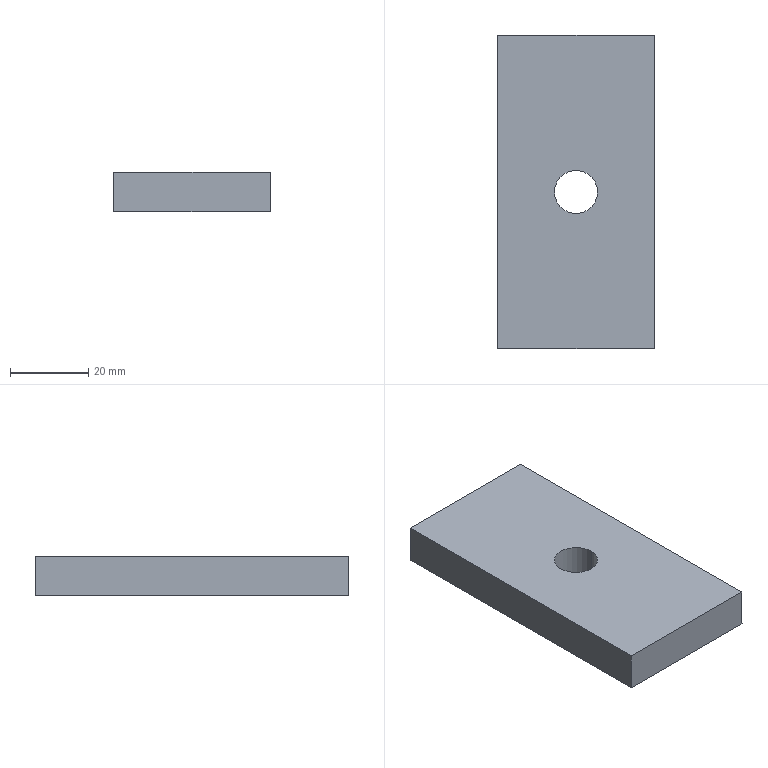Part | SolidWorks | features Extrusion 1, HoleWzd 1 | 1 solid | 8 faces | box 40 x 80 x 10 mm | volume 31050 mm3 | plane 6 | cylinder 2 | commonest cylinder face diameters 11 x2
STEP:
#1=CARTESIAN_POINT('',(14.5,40.,0.));
#2=VERTEX_POINT('',#1);
#3=CARTESIAN_POINT('',(25.5,40.,0.));
#4=VERTEX_POINT('',#3);
#5=CARTESIAN_POINT('',(20.,40.,0.));
#6=DIRECTION('',(0.,0.,1.));
#7=DIRECTION('',(1.,0.,0.));
#8=AXIS2_PLACEMENT_3D('',#5,#6,#7);
#9=CIRCLE('',#8,5.5);
#10=EDGE_CURVE('',#2,#4,#9,.T.);
#11=ORIENTED_EDGE('',*,*,#10,.F.);
#12=CARTESIAN_POINT('',(14.5,40.,10.));
#13=VERTEX_POINT('',#12);
#14=CARTESIAN_POINT('',(14.5,40.,10.));
#15=DIRECTION('',(0.,0.,1.));
#16=VECTOR('',#15,1000.);
#17=LINE('',#14,#16);
#18=EDGE_CURVE('',#2,#13,#17,.T.);
#19=ORIENTED_EDGE('',*,*,#18,.T.);
#20=CARTESIAN_POINT('',(25.5,40.,10.));
#21=VERTEX_POINT('',#20);
#22=CARTESIAN_POINT('',(20.,40.,10.));
#23=DIRECTION('',(0.,0.,1.));
#24=DIRECTION('',(1.,0.,0.));
#25=AXIS2_PLACEMENT_3D('',#22,#23,#24);
#26=CIRCLE('',#25,5.5);
#27=EDGE_CURVE('',#13,#21,#26,.T.);
#28=ORIENTED_EDGE('',*,*,#27,.T.);
#29=CARTESIAN_POINT('',(25.5,40.,10.));
#30=DIRECTION('',(0.,0.,1.));
#31=VECTOR('',#30,1000.);
#32=LINE('',#29,#31);
#33=EDGE_CURVE('',#4,#21,#32,.T.);
#34=ORIENTED_EDGE('',*,*,#33,.F.);
#35=EDGE_LOOP('',(#11,#19,#28,#34));
#36=FACE_OUTER_BOUND('',#35,.T.);
#37=CARTESIAN_POINT('',(20.,40.,10.));
#38=DIRECTION('',(0.,0.,1.));
#39=DIRECTION('',(1.,0.,0.));
#40=AXIS2_PLACEMENT_3D('',#37,#38,#39);
#41=CYLINDRICAL_SURFACE('',#40,5.5);
#42=ADVANCED_FACE('',(#36),#41,.F.);
#43=CARTESIAN_POINT('',(0.,80.,0.));
#44=VERTEX_POINT('',#43);
#45=CARTESIAN_POINT('',(0.,0.,0.));
#46=VERTEX_POINT('',#45);
#47=CARTESIAN_POINT('',(0.,0.,0.));
#48=DIRECTION('',(0.,-1.,0.));
#49=VECTOR('',#48,1000.);
#50=LINE('',#47,#49);
#51=EDGE_CURVE('',#44,#46,#50,.T.);
#52=ORIENTED_EDGE('',*,*,#51,.T.);
#53=CARTESIAN_POINT('',(0.,0.,10.));
#54=VERTEX_POINT('',#53);
#55=CARTESIAN_POINT('',(0.,0.,10.));
#56=DIRECTION('',(0.,0.,-1.));
#57=VECTOR('',#56,1000.);
#58=LINE('',#55,#57);
#59=EDGE_CURVE('',#54,#46,#58,.T.);
#60=ORIENTED_EDGE('',*,*,#59,.F.);
#61=CARTESIAN_POINT('',(0.,80.,10.));
#62=VERTEX_POINT('',#61);
#63=CARTESIAN_POINT('',(0.,0.,10.));
#64=DIRECTION('',(0.,-1.,0.));
#65=VECTOR('',#64,1000.);
#66=LINE('',#63,#65);
#67=EDGE_CURVE('',#62,#54,#66,.T.);
#68=ORIENTED_EDGE('',*,*,#67,.F.);
#69=CARTESIAN_POINT('',(0.,80.,10.));
#70=DIRECTION('',(0.,0.,-1.));
#71=VECTOR('',#70,1000.);
#72=LINE('',#69,#71);
#73=EDGE_CURVE('',#62,#44,#72,.T.);
#74=ORIENTED_EDGE('',*,*,#73,.T.);
#75=EDGE_LOOP('',(#52,#60,#68,#74));
#76=FACE_OUTER_BOUND('',#75,.T.);
#77=CARTESIAN_POINT('',(0.,0.,10.));
#78=DIRECTION('',(1.,0.,0.));
#79=DIRECTION('',(0.,1.,0.));
#80=AXIS2_PLACEMENT_3D('',#77,#78,#79);
#81=PLANE('',#80);
#82=ADVANCED_FACE('',(#76),#81,.F.);
#83=CARTESIAN_POINT('',(40.,0.,0.));
#84=VERTEX_POINT('',#83);
#85=CARTESIAN_POINT('',(0.,0.,0.));
#86=DIRECTION('',(1.,0.,0.));
#87=VECTOR('',#86,1000.);
#88=LINE('',#85,#87);
#89=EDGE_CURVE('',#46,#84,#88,.T.);
#90=ORIENTED_EDGE('',*,*,#89,.T.);
#91=CARTESIAN_POINT('',(40.,0.,10.));
#92=VERTEX_POINT('',#91);
#93=CARTESIAN_POINT('',(40.,0.,10.));
#94=DIRECTION('',(0.,0.,-1.));
#95=VECTOR('',#94,1000.);
#96=LINE('',#93,#95);
#97=EDGE_CURVE('',#92,#84,#96,.T.);
#98=ORIENTED_EDGE('',*,*,#97,.F.);
#99=CARTESIAN_POINT('',(0.,0.,10.));
#100=DIRECTION('',(1.,0.,0.));
#101=VECTOR('',#100,1000.);
#102=LINE('',#99,#101);
#103=EDGE_CURVE('',#54,#92,#102,.T.);
#104=ORIENTED_EDGE('',*,*,#103,.F.);
#105=ORIENTED_EDGE('',*,*,#59,.T.);
#106=EDGE_LOOP('',(#90,#98,#104,#105));
#107=FACE_OUTER_BOUND('',#106,.T.);
#108=CARTESIAN_POINT('',(0.,0.,10.));
#109=DIRECTION('',(0.,1.,0.));
#110=DIRECTION('',(0.,0.,1.));
#111=AXIS2_PLACEMENT_3D('',#108,#109,#110);
#112=PLANE('',#111);
#113=ADVANCED_FACE('',(#107),#112,.F.);
#114=CARTESIAN_POINT('',(40.,80.,0.));
#115=VERTEX_POINT('',#114);
#116=CARTESIAN_POINT('',(40.,0.,0.));
#117=DIRECTION('',(0.,1.,0.));
#118=VECTOR('',#117,1000.);
#119=LINE('',#116,#118);
#120=EDGE_CURVE('',#84,#115,#119,.T.);
#121=ORIENTED_EDGE('',*,*,#120,.T.);
#122=CARTESIAN_POINT('',(40.,80.,10.));
#123=VERTEX_POINT('',#122);
#124=CARTESIAN_POINT('',(40.,80.,10.));
#125=DIRECTION('',(0.,0.,-1.));
#126=VECTOR('',#125,1000.);
#127=LINE('',#124,#126);
#128=EDGE_CURVE('',#123,#115,#127,.T.);
#129=ORIENTED_EDGE('',*,*,#128,.F.);
#130=CARTESIAN_POINT('',(40.,0.,10.));
#131=DIRECTION('',(0.,1.,0.));
#132=VECTOR('',#131,1000.);
#133=LINE('',#130,#132);
#134=EDGE_CURVE('',#92,#123,#133,.T.);
#135=ORIENTED_EDGE('',*,*,#134,.F.);
#136=ORIENTED_EDGE('',*,*,#97,.T.);
#137=EDGE_LOOP('',(#121,#129,#135,#136));
#138=FACE_OUTER_BOUND('',#137,.T.);
#139=CARTESIAN_POINT('',(40.,0.,10.));
#140=DIRECTION('',(-1.,0.,0.));
#141=DIRECTION('',(0.,0.,1.));
#142=AXIS2_PLACEMENT_3D('',#139,#140,#141);
#143=PLANE('',#142);
#144=ADVANCED_FACE('',(#138),#143,.F.);
#145=CARTESIAN_POINT('',(0.,80.,0.));
#146=DIRECTION('',(-1.,0.,0.));
#147=VECTOR('',#146,1000.);
#148=LINE('',#145,#147);
#149=EDGE_CURVE('',#115,#44,#148,.T.);
#150=ORIENTED_EDGE('',*,*,#149,.T.);
#151=ORIENTED_EDGE('',*,*,#73,.F.);
#152=CARTESIAN_POINT('',(0.,80.,10.));
#153=DIRECTION('',(-1.,0.,0.));
#154=VECTOR('',#153,1000.);
#155=LINE('',#152,#154);
#156=EDGE_CURVE('',#123,#62,#155,.T.);
#157=ORIENTED_EDGE('',*,*,#156,.F.);
#158=ORIENTED_EDGE('',*,*,#128,.T.);
#159=EDGE_LOOP('',(#150,#151,#157,#158));
#160=FACE_OUTER_BOUND('',#159,.T.);
#161=CARTESIAN_POINT('',(0.,80.,10.));
#162=DIRECTION('',(0.,-1.,0.));
#163=DIRECTION('',(0.,0.,-1.));
#164=AXIS2_PLACEMENT_3D('',#161,#162,#163);
#165=PLANE('',#164);
#166=ADVANCED_FACE('',(#160),#165,.F.);
#167=CARTESIAN_POINT('',(20.,40.,10.));
#168=DIRECTION('',(0.,0.,1.));
#169=DIRECTION('',(1.,0.,0.));
#170=AXIS2_PLACEMENT_3D('',#167,#168,#169);
#171=CIRCLE('',#170,5.5);
#172=EDGE_CURVE('',#21,#13,#171,.T.);
#173=ORIENTED_EDGE('',*,*,#172,.F.);
#174=ORIENTED_EDGE('',*,*,#27,.F.);
#175=EDGE_LOOP('',(#173,#174));
#176=FACE_BOUND('',#175,.T.);
#177=ORIENTED_EDGE('',*,*,#67,.T.);
#178=ORIENTED_EDGE('',*,*,#103,.T.);
#179=ORIENTED_EDGE('',*,*,#134,.T.);
#180=ORIENTED_EDGE('',*,*,#156,.T.);
#181=EDGE_LOOP('',(#177,#178,#179,#180));
#182=FACE_OUTER_BOUND('',#181,.T.);
#183=CARTESIAN_POINT('',(0.,0.,10.));
#184=DIRECTION('',(0.,0.,-1.));
#185=DIRECTION('',(-1.,0.,0.));
#186=AXIS2_PLACEMENT_3D('',#183,#184,#185);
#187=PLANE('',#186);
#188=ADVANCED_FACE('',(#176,#182),#187,.F.);
#189=CARTESIAN_POINT('',(20.,40.,0.));
#190=DIRECTION('',(0.,0.,1.));
#191=DIRECTION('',(1.,0.,0.));
#192=AXIS2_PLACEMENT_3D('',#189,#190,#191);
#193=CIRCLE('',#192,5.5);
#194=EDGE_CURVE('',#4,#2,#193,.T.);
#195=ORIENTED_EDGE('',*,*,#194,.T.);
#196=ORIENTED_EDGE('',*,*,#10,.T.);
#197=EDGE_LOOP('',(#195,#196));
#198=FACE_BOUND('',#197,.T.);
#199=ORIENTED_EDGE('',*,*,#51,.F.);
#200=ORIENTED_EDGE('',*,*,#149,.F.);
#201=ORIENTED_EDGE('',*,*,#120,.F.);
#202=ORIENTED_EDGE('',*,*,#89,.F.);
#203=EDGE_LOOP('',(#199,#200,#201,#202));
#204=FACE_OUTER_BOUND('',#203,.T.);
#205=CARTESIAN_POINT('',(0.,0.,0.));
#206=DIRECTION('',(0.,0.,-1.));
#207=DIRECTION('',(-1.,0.,0.));
#208=AXIS2_PLACEMENT_3D('',#205,#206,#207);
#209=PLANE('',#208);
#210=ADVANCED_FACE('',(#198,#204),#209,.T.);
#211=ORIENTED_EDGE('',*,*,#18,.F.);
#212=ORIENTED_EDGE('',*,*,#194,.F.);
#213=ORIENTED_EDGE('',*,*,#33,.T.);
#214=ORIENTED_EDGE('',*,*,#172,.T.);
#215=EDGE_LOOP('',(#211,#212,#213,#214));
#216=FACE_OUTER_BOUND('',#215,.T.);
#217=CARTESIAN_POINT('',(20.,40.,10.));
#218=DIRECTION('',(0.,0.,1.));
#219=DIRECTION('',(1.,0.,0.));
#220=AXIS2_PLACEMENT_3D('',#217,#218,#219);
#221=CYLINDRICAL_SURFACE('',#220,5.5);
#222=ADVANCED_FACE('',(#216),#221,.F.);
#223=CLOSED_SHELL('',(#42,#82,#113,#144,#166,#188,#210,#222));
#224=MANIFOLD_SOLID_BREP('',#223);
#225=CARTESIAN_POINT('',(0.,0.,0.));
#226=DIRECTION('',(0.,0.,1.));
#227=DIRECTION('',(1.,0.,0.));
#228=AXIS2_PLACEMENT_3D('',#225,#226,#227);
#229=(LENGTH_UNIT()NAMED_UNIT(*)SI_UNIT(.MILLI.,.METRE.));
#230=UNCERTAINTY_MEASURE_WITH_UNIT(LENGTH_MEASURE(0.00001),#229,'','');
#231=(NAMED_UNIT(*)PLANE_ANGLE_UNIT()SI_UNIT($,.RADIAN.));
#232=(NAMED_UNIT(*)SI_UNIT($,.STERADIAN.)SOLID_ANGLE_UNIT());
#233=(GEOMETRIC_REPRESENTATION_CONTEXT(3)GLOBAL_UNCERTAINTY_ASSIGNED_CONTEXT((#230))GLOBAL_UNIT_ASSIGNED_CONTEXT((#229,#231,#232))REPRESENTATION_CONTEXT('',''));
#234=ADVANCED_BREP_SHAPE_REPRESENTATION('',(#224,#228),#233);